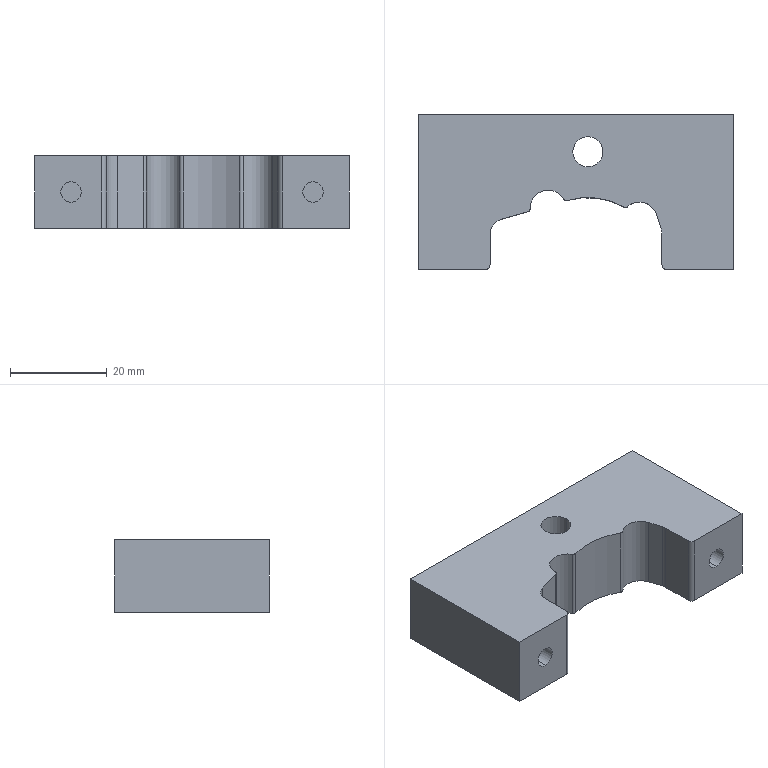NC program | Mastercam | posted with a generic post
Lines 1461 to 2481 of 2481:
N4690 T3 M6
N4700 G0 G90 G17 G54 X-12. Y-7.93 A0. S5500 M3
N4710 G43 H3 Z50.
N4720 Z2.
N4730 G1 Z-7.75 F2000.
N4740 X-12.829 Y-7.749 Z-7.901 F1500.
N4750 G3 X-13.069 Y-7.723 Z-7.944 I-.24 J-1.099
N4760 X-13.378 Y-7.766 Z-8. I0. J-1.125
N4770 G1 X-13.645 Y-7.842
N4780 G3 X-14.94 Y-8.789 I.372 J-1.868
N4790 X-15.116 Y-9.152 I2.014 J-1.201
N4800 X-15.15 Y-9.333 I.466 J-.181
N4810 G1 Y-9.519
N4820 Y-9.704
N4830 G3 X-14.22 Y-10.812 Z-7.75 I1.125 J0.
N4840 X-14.025 Y-10.829 I.195 J1.108 F9500.
N4850 X-13.15 Y-10.411 I0. J1.125
N4860 G1 X-12.537 Y-9.653
N4870 G3 X-12.287 Y-8.946 I-.875 J.707
N4880 X-12.4 Y-8.454 I-1.125 J0.
N4890 X-13.412 Y-7.821 Z-7.95 I-1.012 J-.492 F1500.
N4900 X-13.72 Y-7.864 Z-8. I0. J-1.125
N4910 G1 X-13.987 Y-7.94
N4920 G3 X-14.983 Y-8.648 I.375 J-1.582
N4930 X-15.088 Y-8.819 I1.467 J-1.022
N4940 X-15.15 Y-9.06 I.438 J-.241
N4950 G1 Y-9.245
N4960 Y-9.616
N4970 G3 X-14.22 Y-10.723 Z-7.75 I1.125 J0.
N4980 X-14.025 Y-10.74 I.195 J1.107 F9500.
N4990 X-13.102 Y-10.259 I0. J1.124
N5000 G1 X-12.671 Y-9.641
N5010 G3 X-12.469 Y-8.998 I-.923 J.643
N5020 X-12.582 Y-8.506 I-1.125 J0.
N5030 X-13.594 Y-7.873 Z-7.95 I-1.012 J-.492 F1500.
N5040 X-13.902 Y-7.916 Z-8. I0. J-1.125
N5050 G1 X-14.17 Y-7.992
N5060 G3 X-15.062 Y-8.589 I.257 J-1.348
N5070 X-15.15 Y-8.873 I.412 J-.284
N5080 G1 Y-9.058
N5090 Y-9.243
N5100 G3 X-14.22 Y-10.351 Z-7.75 I1.125 J0.
N5110 X-14.025 Y-10.368 I.195 J1.108 F9500.
N5120 X-13.265 Y-10.073 I0. J1.125
N5130 G1 X-13.07 Y-9.894
N5140 G3 X-12.705 Y-9.065 I-.76 J.829
N5150 X-12.819 Y-8.574 I-1.125 J0.
N5160 X-13.83 Y-7.941 Z-7.95 I-1.011 J-.491 F1500.
N5170 X-14.139 Y-7.983 Z-8. I0. J-1.124
N5180 G1 X-14.406 Y-8.059
N5190 G3 X-15.025 Y-8.412 I.199 J-1.068
N5200 X-15.15 Y-8.744 I.375 J-.332
N5210 G1 Y-8.929
N5220 Y-9.114
N5230 G3 X-14.22 Y-10.222 Z-7.75 I1.125 J0.
N5240 X-14.141 Y-10.233 I.195 J1.108 F9500.
N5250 X-14.009 Y-10.241 I.132 J1.117
N5260 X-12.884 Y-9.116 I0. J1.125
N5270 X-12.997 Y-8.624 I-1.125 J0.
N5280 X-14.009 Y-7.991 Z-7.95 I-1.012 J-.492 F1500.
N5290 X-14.317 Y-8.034 Z-8. I0. J-1.125
N5300 G1 X-14.584 Y-8.11
N5310 G3 X-14.882 Y-8.225 I.218 J-1.014
N5320 X-15.15 Y-8.724 I.332 J-.499
N5330 G1 Y-8.91
N5340 G3 X-14.22 Y-10.018 Z-7.75 I1.125 J0.
N5350 X-14.025 Y-10.035 I.195 J1.108 F9500.
N5360 X-13.603 Y-9.953 I0. J1.125
N5370 G1 X-3.746 Y-5.968
N5380 G3 X-3.109 Y-5.305 I-.422 J1.043
N5390 X-3.043 Y-4.925 Z-7.812 I-1.059 J.38 F1500.
N5400 X-3.61 Y-3.948 Z-8. I-1.125 J0.
N5410 G2 X-4.135 Y-3.586 I2.23 J3.793
N5420 G3 X-5.145 Y-3.338 I-1.01 J-1.933
N5430 X-5.937 Y-3.486 I0. J-2.181
N5440 X-6.878 Y-4.133 I.851 J-2.249
N5450 X-6.992 Y-4.334 I.366 J-.34
N5460 G2 X-7.049 Y-4.511 I-3.171 J.916
N5470 G3 X-7.112 Y-4.883 Z-7.94 I1.062 J-.372
N5480 X-6.538 Y-5.864 Z-7.75 I1.125 J0.
N5490 X-5.987 Y-6.008 I.551 J.981 F9500.
N5500 X-5.857 Y-6.001 I0. J1.125
N5510 G1 X-4.376 Y-5.829
N5520 G3 X-3.485 Y-5.185 I-.129 J1.118
N5530 X-3.38 Y-4.711 Z-7.828 I-1.02 J.474 F1500.
N5540 X-3.861 Y-3.789 Z-8. I-1.125 J0.
N5550 G2 X-4.262 Y-3.468 I1.729 J2.577
N5560 G3 X-5.198 Y-3.223 I-.936 J-1.662
N5570 X-5.612 Y-3.269 I0. J-1.907
N5580 X-6.806 Y-3.886 I.46 J-2.353
N5590 X-6.94 Y-4.131 I.354 J-.353
N5600 G2 X-6.986 Y-4.311 I-3.223 J.713
N5610 G3 X-7.028 Y-4.615 Z-7.951 I1.083 J-.304
N5620 X-6.39 Y-5.629 Z-7.75 I1.125 J0.
N5630 X-5.903 Y-5.74 I.487 J1.014 F9500.
N5640 X-5.854 Y-5.739 I0. J1.125
N5650 G1 X-4.656 Y-5.687
N5660 G3 X-3.713 Y-5.094 I-.049 J1.124
N5670 X-3.58 Y-4.563 Z-7.838 I-.992 J.531 F1500.
N5680 X-4.01 Y-3.679 Z-8. I-1.125 J0.
N5690 G2 X-4.397 Y-3.338 I2.158 J2.843
N5700 G3 X-5.27 Y-3.118 I-.873 J-1.622
N5710 X-5.649 Y-3.157 I0. J-1.842
N5720 X-6.76 Y-3.691 I.388 J-2.23
N5730 X-6.909 Y-3.97 I.344 J-.363
N5740 G2 X-6.945 Y-4.152 I-3.254 J.552
N5750 G3 X-6.973 Y-4.402 Z-7.96 I1.097 J-.25
N5760 X-6.285 Y-5.439 Z-7.75 I1.125 J0.
N5770 X-5.851 Y-5.527 I.437 J1.037 F9500.
N5780 G1 X-4.899 Y-5.529
N5790 X-4.896
N5800 G3 X-3.935 Y-4.99 I0. J1.125
N5810 X-3.77 Y-4.404 Z-7.848 I-.961 J.586 F1500.
N5820 X-4.153 Y-3.56 Z-8. I-1.126 J0.
N5830 G2 X-4.471 Y-3.252 I2.329 J2.723
N5840 G1 X-4.513 Y-3.224
N5850 G3 X-5.341 Y-3.014 I-.828 J-1.531
N5860 X-5.658 Y-3.043 I0. J-1.741
N5870 X-6.734 Y-3.528 I.277 J-2.05
N5880 X-6.888 Y-3.831 I.342 J-.365
N5890 G2 X-6.917 Y-4.014 I-3.275 J.413
N5900 G3 X-6.935 Y-4.217 Z-7.968 I1.107 J-.203
N5910 X-6.202 Y-5.271 Z-7.75 I1.125 J0.
N5920 X-5.922 Y-5.336 I.392 J1.054 F9500.
N5930 G1 X-5.126 Y-5.415
N5940 G3 X-5.015 Y-5.42 I.111 J1.119
N5950 X-4.076 Y-4.916 I0. J1.124
N5960 X-3.89 Y-4.296 Z-7.854 I-.939 J.62 F1500.
N5970 X-4.241 Y-3.479 Z-8. I-1.125 J0.
N5980 G2 X-4.55 Y-3.158 I2.414 J2.626
N5990 G1 X-4.589 Y-3.13
N6000 G3 X-5.415 Y-2.912 I-.826 J-1.456
N6010 X-5.699 Y-2.936 I0. J-1.674
N6020 X-6.722 Y-3.386 I.209 J-1.863
N6030 X-6.875 Y-3.705 I.345 J-.362
N6040 G2 X-6.928 Y-4.071 I-3.288 J.287
N6050 G3 X-6.95 Y-4.294 Z-7.964 I1.103 J-.223
N6060 X-6.236 Y-5.341 Z-7.75 I1.125 J0.
N6070 X-5.825 Y-5.419 I.411 J1.047 F9500.
N6080 X-5.64 Y-5.404 I0. J1.125
N6090 G1 X-4.949 Y-5.288
N6100 G3 X-4.219 Y-4.834 I-.185 J1.109
N6110 X-4.009 Y-4.179 Z-7.861 I-.915 J.655 F1500.
N6120 X-4.33 Y-3.392 Z-8. I-1.125 J0.
N6130 G2 X-4.614 Y-3.074 I2.538 J2.551
N6140 G1 X-4.65 Y-3.046
N6150 G3 X-5.482 Y-2.811 I-.832 J-1.356
N6160 X-5.721 Y-2.829 I0. J-1.591
N6170 X-6.712 Y-3.252 I.153 J-1.731
N6180 X-6.867 Y-3.589 I.344 J-.362
N6190 G2 X-6.907 Y-3.957 I-3.296 J.171
N6200 G3 X-6.922 Y-4.14 Z-7.971 I1.11 J-.183
N6210 X-6.17 Y-5.202 Z-7.75 I1.125 J0.
N6220 X-5.797 Y-5.266 I.373 J1.062 F9500.
N6230 X-5.663 Y-5.257 I0. J1.126
N6240 G1 X-5.1 Y-5.19
N6250 G3 X-4.342 Y-4.758 I-.134 J1.117
N6260 X-4.109 Y-4.073 Z-7.867 I-.892 J.685 F1500.
N6270 X-4.405 Y-3.313 Z-8. I-1.125 J0.
N6280 G2 X-4.677 Y-2.987 I2.534 J2.394
N6290 G1 X-4.711 Y-2.959
N6300 G3 X-5.544 Y-2.711 I-.833 J-1.276
N6310 X-5.747 Y-2.725 I0. J-1.524
N6320 X-6.723 Y-3.143 I.113 J-1.611
N6330 X-6.863 Y-3.481 I.36 J-.347
N6340 G2 X-6.891 Y-3.85 I-3.3 J.063
N6350 G3 X-6.901 Y-3.997 Z-7.977 I1.115 J-.147
N6360 X-6.114 Y-5.07 Z-7.75 I1.125 J0.
N6370 X-5.776 Y-5.122 I.338 J1.073 F9500.
N6380 X-5.693 Y-5.119 I0. J1.125
N6390 G1 X-5.247 Y-5.086
N6400 G3 X-4.461 Y-4.678 I-.083 J1.122
N6410 X-4.205 Y-3.964 Z-7.873 I-.869 J.714 F1500.
N6420 X-4.477 Y-3.232 Z-8. I-1.125 J0.
N6430 G2 X-4.733 Y-2.904 I2.56 J2.266
N6440 G1 X-4.765 Y-2.876
N6450 G3 X-5.614 Y-2.613 I-.849 J-1.239
N6460 X-5.849 Y-2.631 I0. J-1.502
N6470 X-6.721 Y-3.024 I.14 J-1.476
N6480 X-6.863 Y-3.373 I.358 J-.349
N6490 G1 Y-3.379
N6500 Y-3.418
N6510 G2 X-6.879 Y-3.749 I-3.3 J0.
N6520 G3 X-6.885 Y-3.861 Z-7.982 I1.119 J-.112
N6530 X-6.065 Y-4.944 Z-7.75 I1.125 J0.
N6540 X-5.76 Y-4.986 I.305 J1.083 F9500.
N6550 G1 X-5.754
N6560 X-5.412 Y-4.985
N6570 G3 X-4.57 Y-4.6 I-.005 J1.125
N6580 X-4.292 Y-3.86 Z-7.879 I-.847 J.74 F1500.
N6590 X-4.541 Y-3.154 Z-8. I-1.125 J0.
N6600 G2 X-4.786 Y-2.82 I2.721 J2.255
N6610 G1 X-4.817 Y-2.792
N6620 X-5.046 Y-2.648
N6630 G3 X-5.675 Y-2.519 I-.629 J-1.472
N6640 X-6.716 Y-2.904 I0. J-1.601
N6650 X-6.858 Y-3.206 I.355 J-.352
N6660 X-6.863 Y-3.315 I1.094 J-.109
N6670 G1 Y-3.341
N6680 G2 X-6.862 Y-3.418 I-3.3 J-.077
N6690 X-6.864 Y-3.526 I-3.301 J0.
N6700 G3 X-6.865 Y-3.563 Z-7.994 I1.124 J-.037
N6710 X-6.441 Y-4.443 Z-7.833 I1.125 J0.
N6720 G1 X-6.201 Y-4.634 Z-7.784
N6730 G3 X-6.019 Y-4.752 Z-7.75 I.701 J.88
N6740 X-5.5 Y-4.879 I.519 J.998 F9500.
N6750 X-4.675 Y-4.52 I0. J1.125
N6760 X-4.374 Y-3.754 Z-7.884 I-.825 J.766 F1500.
N6770 X-4.603 Y-3.075 Z-8. I-1.126 J0.
N6780 G2 X-4.835 Y-2.738 I2.854 J2.214
N6790 G1 X-4.864 Y-2.71
N6800 X-5.083 Y-2.564
N6810 G3 X-5.725 Y-2.426 I-.642 J-1.421
N6820 X-6.639 Y-2.721 I0. J-1.559
N6830 X-6.8 Y-2.946 I.31 J-.393
N6840 X-6.864 Y-3.315 I1.036 J-.369
N6850 X-6.863 Y-3.341 I1.1 J0.
N6860 G2 X-6.862 Y-3.418 I-3.3 J-.077
N6870 X-6.864 Y-3.526 I-3.301 J0.
N6880 G3 X-6.865 Y-3.563 Z-7.994 I1.124 J-.037
N6890 X-6.268 Y-4.556 Z-7.8 I1.125 J0.
N6900 G1 X-6.104 Y-4.643 Z-7.771
N6910 G3 X-5.985 Y-4.698 Z-7.75 I.528 J.993
N6920 X-5.576 Y-4.775 I.409 J1.048 F9500.
N6930 X-4.775 Y-4.439 I0. J1.125
N6940 X-4.452 Y-3.65 Z-7.889 I-.801 J.789 F1500.
N6950 X-4.66 Y-2.997 Z-8. I-1.124 J0.
N6960 G2 X-4.816 Y-2.757 I2.688 J1.914
N6970 G3 X-4.893 Y-2.643 I-.948 J-.558
N6980 G1 X-4.923 Y-2.614
N6990 X-5.146 Y-2.466
N7000 G3 X-5.77 Y-2.333 I-.624 J-1.393
N7010 X-6.46 Y-2.497 I0. J-1.526
N7020 X-6.627 Y-2.633 I.225 J-.446
N7030 X-6.849 Y-3.137 I.863 J-.682
N7040 X-6.862 Y-3.294 Z-7.975 I.956 J-.157
N7050 X-6.836 Y-3.517 Z-7.939 I.969 J0.
N7060 G1 X-6.782 Y-3.747 Z-7.901
N7070 G3 X-6.219 Y-4.479 Z-7.75 I1.095 J.26
N7080 X-5.687 Y-4.613 I.532 J.992 F9500.
N7090 X-4.921 Y-4.311 I0. J1.126
N7100 X-4.562 Y-3.487 Z-7.897 I-.766 J.824 F1500.
N7110 X-4.742 Y-2.876 Z-8. I-1.125 J0.
N7120 G2 X-4.816 Y-2.757 I2.77 J1.793
N7130 G3 X-5.118 Y-2.428 I-.891 J-.517
N7140 G1 X-5.163 Y-2.401
N7150 G3 X-5.801 Y-2.242 I-.638 J-1.204
N7160 X-6.174 Y-2.295 I0. J-1.363
N7170 X-6.721 Y-2.774 I.41 J-1.02
N7180 X-6.847 Y-3.251 Z-7.921 I.843 J-.477
N7190 X-6.311 Y-4.117 Z-7.75 I.969 J0.
N7200 X-5.878 Y-4.219 I.433 J.866 F9500.
N7210 X-5.834 Y-4.218 I0. J.968
N7220 X-5.757 Y-4.22 I.077 J1.271
N7230 X-5.146 Y-4.064 I0. J1.273
N7240 X-4.688 Y-3.241 Z-7.907 I-.51 J.823 F1500.
N7250 X-4.859 Y-2.69 Z-8. I-.968 J0.
N7260 X-5.764 Y-2.215 I-.905 J-.625
N7270 X-6.416 Y-2.429 I0. J-1.1
N7280 X-6.811 Y-3.21 Z-7.856 I.574 J-.781
N7290 X-6.592 Y-3.822 Z-7.75 I.969 J0.
N7300 X-6.051 Y-4.155 I.75 J.612 F9500.
N7310 G1 X13.364 Y-8.459
N7320 G3 X13.608 Y-8.486 I.244 J1.099
N7330 X14.133 Y-8.356 I0. J1.126
N7340 X14.734 Y-7.36 Z-7.944 I-.525 J.996 F1500.
N7350 X14.679 Y-7.016 Z-8. I-1.126 J0.
N7360 G1 X14.594 Y-6.752
N7370 G3 X13.611 Y-5.488 I-1.862 J-.434
N7380 X12.415 Y-5.199 I-1.196 J-2.332
N7390 X12.173 Y-5.21 I0. J-2.621
N7400 X11.96 Y-5.283 I.05 J-.498
N7410 G2 X11.8 Y-5.376 I-1.735 J2.807
N7420 G3 X11.212 Y-6.364 Z-7.808 I.537 J-.988
N7430 X11.27 Y-6.721 Z-7.75 I1.125 J0.
N7440 X11.783 Y-7.343 I1.067 J.357 F9500.
N7450 G1 X12.945 Y-8.
N7460 G3 X13.499 Y-8.146 I.554 J.979
N7470 X14.024 Y-8.016 I0. J1.125
N7480 X14.624 Y-7.021 Z-7.944 I-.525 J.995 F1500.
N7490 X14.57 Y-6.677 Z-8. I-1.125 J0.
N7500 G1 X14.485 Y-6.412
N7510 G3 X13.738 Y-5.433 I-1.574 J-.426
N7520 X12.456 Y-5.073 I-1.282 J-2.106
N7530 X12.409 Y-5.074 I0. J-2.466
N7540 X12.136 Y-5.166 I.016 J-.5
N7550 G2 X11.982 Y-5.269 I-1.911 J2.69
N7560 G3 X11.455 Y-6.222 Z-7.819 I.599 J-.953
N7570 X11.539 Y-6.646 Z-7.75 I1.126 J0.
N7580 X11.928 Y-7.138 I1.042 J.424 F9500.
N7590 G1 X12.786 Y-7.748
N7600 G3 X13.438 Y-7.956 I.652 J.916
N7610 X13.963 Y-7.827 I0. J1.124
N7620 X14.563 Y-6.832 Z-7.944 I-.525 J.995 F1500.
N7630 X14.509 Y-6.488 Z-8. I-1.125 J0.
N7640 G1 X14.424 Y-6.223
N7650 G3 X13.735 Y-5.309 I-1.403 J-.341
N7660 X12.566 Y-4.961 I-1.184 J-1.843
N7670 X12.267 Y-5.068 I.01 J-.5
N7680 G2 X12.118 Y-5.179 I-2.042 J2.592
N7690 G3 X11.639 Y-6.1 Z-7.828 I.645 J-.921
N7700 X11.744 Y-6.576 Z-7.75 I1.124 J0.
N7710 X12.04 Y-6.962 I1.019 J.476 F9500.
N7720 G1 X12.642 Y-7.468
N7730 G3 X13.365 Y-7.731 I.723 J.862
N7740 X13.89 Y-7.601 I0. J1.125
N7750 X14.49 Y-6.606 Z-7.944 I-.525 J.995 F1500.
N7760 X14.437 Y-6.262 Z-8. I-1.125 J0.
N7770 G1 X14.352 Y-5.997
N7780 G3 X13.769 Y-5.213 I-1.278 J-.341
N7790 X12.69 Y-4.86 I-1.11 J-1.569
N7800 X12.373 Y-4.98 I.009 J-.5
N7810 G2 X12.23 Y-5.097 I-2.148 J2.504
N7820 G3 X11.788 Y-5.991 Z-7.836 I.683 J-.894
N7830 X11.914 Y-6.509 Z-7.75 I1.125 J0.
N7840 X12.078 Y-6.744 I.999 J.518 F9500.
N7850 G1 X12.473 Y-7.183
N7860 G3 X13.309 Y-7.555 I.836 J.753
N7870 X13.834 Y-7.425 I0. J1.125
N7880 X14.434 Y-6.43 Z-7.944 I-.525 J.995 F1500.
N7890 X14.38 Y-6.086 Z-8. I-1.125 J0.
N7900 G1 X14.295 Y-5.821
N7910 G3 X14.143 Y-5.468 I-.983 J-.213
N7920 X12.837 Y-4.766 I-1.415 J-1.067
N7930 G1 X12.823
N7940 G3 X12.569 Y-4.835 I0. J-.5
N7950 X12.402 Y-4.956 I.558 J-.948
N7960 G2 X12.259 Y-5.074 I-2.177 J2.48
N7970 G3 X11.828 Y-5.96 Z-7.838 I.694 J-.886
N7980 X11.96 Y-6.489 Z-7.75 I1.125 J0.
N7990 X12.166 Y-6.764 I.993 J.529 F9500.
N8000 G1 X12.465 Y-7.057
N8010 G3 X13.252 Y-7.378 I.787 J.804
N8020 X13.777 Y-7.248 I0. J1.125
N8030 X14.377 Y-6.253 Z-7.944 I-.525 J.995 F1500.
N8040 X14.323 Y-5.909 Z-8. I-1.125 J0.
N8050 G1 X14.238 Y-5.645
N8060 X14.138 Y-5.383
N8070 G3 X13.14 Y-4.703 I-1.31 J-.852
N8080 X13.028 Y-4.69 I-.112 J-.488
N8090 X12.946 Y-4.698 I0. J-.501
N8100 X12.402 Y-4.956 I.181 J-1.085
N8110 G2 X12.259 Y-5.074 I-2.177 J2.48
N8120 G3 X11.828 Y-5.96 Z-7.838 I.694 J-.886
N8130 X11.96 Y-6.489 Z-7.75 I1.125 J0.
N8140 X12.465 Y-6.974 I.993 J.529 F9500.
N8150 G1 X12.708 Y-7.091
N8160 G3 X13.196 Y-7.202 I.488 J1.014
N8170 X13.72 Y-7.072 I0. J1.125
N8180 X14.321 Y-6.077 Z-7.944 I-.524 J.995 F1500.
N8190 X14.267 Y-5.733 Z-8. I-1.125 J0.
N8200 G1 X14.182 Y-5.468
N8210 G3 X13.127 Y-4.682 I-1.055 J-.315
N8220 X12.725 Y-4.759 I0. J-1.101
N8230 X12.11 Y-5.661 Z-7.815 I.354 J-.902
N8240 X12.197 Y-6.06 Z-7.75 I.969 J0.
N8250 X12.701 Y-6.553 I.882 J.399 F9500.
N8260 X13.238 Y-6.7 I.537 J.906
N8270 X13.575 Y-6.644 I0. J1.053
N8280 X14.217 Y-5.732 Z-7.939 I-.327 J.912 F1500.
N8290 X14.143 Y-5.359 Z-8. I-.969 J0.
N8300 X13.574 Y-4.777 I-1.016 J-.424
N8310 X13.181 Y-4.694 Z-7.936 I-.393 J-.886
N8320 X12.663 Y-4.844 Z-7.849 I0. J-.969
N8330 G1 X12.139 Y-5.175 Z-7.75
N8340 X10.346 Y-6.309 F9500.
N8350 G0 Z50.
N8360 X-12. Y-7.93
N8370 Z-6.
N8380 G1 Z-15.75 F2000.
N8390 X-12.829 Y-7.749 Z-15.901 F1500.
N8400 G3 X-13.069 Y-7.723 Z-15.944 I-.24 J-1.099
N8410 X-13.378 Y-7.766 Z-16. I0. J-1.125
N8420 G1 X-13.645 Y-7.842
N8430 G3 X-14.94 Y-8.789 I.372 J-1.868
N8440 X-15.116 Y-9.152 I2.014 J-1.201
N8450 X-15.15 Y-9.333 I.466 J-.181
N8460 G1 Y-9.519
N8470 Y-9.704
N8480 G3 X-14.22 Y-10.812 Z-15.75 I1.125 J0.
N8490 X-14.025 Y-10.829 I.195 J1.108 F9500.
N8500 X-13.15 Y-10.411 I0. J1.125
N8510 G1 X-12.537 Y-9.653
N8520 G3 X-12.287 Y-8.946 I-.875 J.707
N8530 X-12.4 Y-8.454 I-1.125 J0.
N8540 X-13.412 Y-7.821 Z-15.95 I-1.012 J-.492 F1500.
N8550 X-13.72 Y-7.864 Z-16. I0. J-1.125
N8560 G1 X-13.987 Y-7.94
N8570 G3 X-14.983 Y-8.648 I.375 J-1.582
N8580 X-15.088 Y-8.819 I1.467 J-1.022
N8590 X-15.15 Y-9.06 I.438 J-.241
N8600 G1 Y-9.245
N8610 Y-9.616
N8620 G3 X-14.22 Y-10.723 Z-15.75 I1.125 J0.
N8630 X-14.025 Y-10.74 I.195 J1.107 F9500.
N8640 X-13.102 Y-10.259 I0. J1.124
N8650 G1 X-12.671 Y-9.641
N8660 G3 X-12.469 Y-8.998 I-.923 J.643
N8670 X-12.582 Y-8.506 I-1.125 J0.
N8680 X-13.594 Y-7.873 Z-15.95 I-1.012 J-.492 F1500.
N8690 X-13.902 Y-7.916 Z-16. I0. J-1.125
N8700 G1 X-14.17 Y-7.992
N8710 G3 X-15.062 Y-8.589 I.257 J-1.348
N8720 X-15.15 Y-8.873 I.412 J-.284
N8730 G1 Y-9.058
N8740 Y-9.243
N8750 G3 X-14.22 Y-10.351 Z-15.75 I1.125 J0.
N8760 X-14.025 Y-10.368 I.195 J1.108 F9500.
N8770 X-13.265 Y-10.073 I0. J1.125
N8780 G1 X-13.07 Y-9.894
N8790 G3 X-12.705 Y-9.065 I-.76 J.829
N8800 X-12.819 Y-8.574 I-1.125 J0.
N8810 X-13.83 Y-7.941 Z-15.95 I-1.011 J-.491 F1500.
N8820 X-14.139 Y-7.983 Z-16. I0. J-1.124
N8830 G1 X-14.406 Y-8.059
N8840 G3 X-15.025 Y-8.412 I.199 J-1.068
N8850 X-15.15 Y-8.744 I.375 J-.332
N8860 G1 Y-8.929
N8870 Y-9.114
N8880 G3 X-14.22 Y-10.222 Z-15.75 I1.125 J0.
N8890 X-14.141 Y-10.233 I.195 J1.108 F9500.
N8900 X-14.009 Y-10.241 I.132 J1.117
N8910 X-12.884 Y-9.116 I0. J1.125
N8920 X-12.997 Y-8.624 I-1.125 J0.
N8930 X-14.009 Y-7.991 Z-15.95 I-1.012 J-.492 F1500.
N8940 X-14.317 Y-8.034 Z-16. I0. J-1.125
N8950 G1 X-14.584 Y-8.11
N8960 G3 X-14.882 Y-8.225 I.218 J-1.014
N8970 X-15.15 Y-8.724 I.332 J-.499
N8980 G1 Y-8.91
N8990 G3 X-14.22 Y-10.018 Z-15.75 I1.125 J0.
N9000 X-14.025 Y-10.035 I.195 J1.108 F9500.
N9010 X-13.603 Y-9.953 I0. J1.125
N9020 G1 X-3.746 Y-5.968
N9030 G3 X-3.109 Y-5.305 I-.422 J1.043
N9040 X-3.043 Y-4.925 Z-15.812 I-1.059 J.38 F1500.
N9050 X-3.61 Y-3.948 Z-16. I-1.125 J0.
N9060 G2 X-4.135 Y-3.586 I2.23 J3.793
N9070 G3 X-5.145 Y-3.338 I-1.01 J-1.933
N9080 X-5.937 Y-3.486 I0. J-2.181
N9090 X-6.878 Y-4.133 I.851 J-2.249
N9100 X-6.992 Y-4.334 I.366 J-.34
N9110 G2 X-7.049 Y-4.511 I-3.171 J.916
N9120 G3 X-7.112 Y-4.883 Z-15.94 I1.062 J-.372
N9130 X-6.538 Y-5.864 Z-15.75 I1.125 J0.
N9140 X-5.987 Y-6.008 I.551 J.981 F9500.
N9150 X-5.857 Y-6.001 I0. J1.125
N9160 G1 X-4.376 Y-5.829
N9170 G3 X-3.485 Y-5.185 I-.129 J1.118
N9180 X-3.38 Y-4.711 Z-15.828 I-1.02 J.474 F1500.
N9190 X-3.861 Y-3.789 Z-16. I-1.125 J0.
N9200 G2 X-4.262 Y-3.468 I1.729 J2.577
N9210 G3 X-5.198 Y-3.223 I-.936 J-1.662
N9220 X-5.612 Y-3.269 I0. J-1.907
N9230 X-6.806 Y-3.886 I.46 J-2.353
N9240 X-6.94 Y-4.131 I.354 J-.353
N9250 G2 X-6.986 Y-4.311 I-3.223 J.713
N9260 G3 X-7.028 Y-4.615 Z-15.951 I1.083 J-.304
N9270 X-6.39 Y-5.629 Z-15.75 I1.125 J0.
N9280 X-5.903 Y-5.74 I.487 J1.014 F9500.
N9290 X-5.854 Y-5.739 I0. J1.125
N9300 G1 X-4.656 Y-5.687
N9310 G3 X-3.713 Y-5.094 I-.049 J1.124
N9320 X-3.58 Y-4.563 Z-15.838 I-.992 J.531 F1500.
N9330 X-4.01 Y-3.679 Z-16. I-1.125 J0.
N9340 G2 X-4.397 Y-3.338 I2.158 J2.843
N9350 G3 X-5.27 Y-3.118 I-.873 J-1.622
N9360 X-5.649 Y-3.157 I0. J-1.842
N9370 X-6.76 Y-3.691 I.388 J-2.23
N9380 X-6.909 Y-3.97 I.344 J-.363
N9390 G2 X-6.945 Y-4.152 I-3.254 J.552
N9400 G3 X-6.973 Y-4.402 Z-15.96 I1.097 J-.25
N9410 X-6.285 Y-5.439 Z-15.75 I1.125 J0.
N9420 X-5.851 Y-5.527 I.437 J1.037 F9500.
N9430 G1 X-4.899 Y-5.529
N9440 X-4.896
N9450 G3 X-3.935 Y-4.99 I0. J1.125
N9460 X-3.77 Y-4.404 Z-15.848 I-.961 J.586 F1500.
N9470 X-4.153 Y-3.56 Z-16. I-1.126 J0.
N9480 G2 X-4.471 Y-3.252 I2.329 J2.723
N9490 G1 X-4.513 Y-3.224
N9500 G3 X-5.341 Y-3.014 I-.828 J-1.531
N9510 X-5.658 Y-3.043 I0. J-1.741
N9520 X-6.734 Y-3.528 I.277 J-2.05
N9530 X-6.888 Y-3.831 I.342 J-.365
N9540 G2 X-6.917 Y-4.014 I-3.275 J.413
N9550 G3 X-6.935 Y-4.217 Z-15.968 I1.107 J-.203
N9560 X-6.202 Y-5.271 Z-15.75 I1.125 J0.
N9570 X-5.922 Y-5.336 I.392 J1.054 F9500.
N9580 G1 X-5.126 Y-5.415
N9590 G3 X-5.015 Y-5.42 I.111 J1.119
N9600 X-4.076 Y-4.916 I0. J1.124
N9610 X-3.89 Y-4.296 Z-15.854 I-.939 J.62 F1500.
N9620 X-4.241 Y-3.479 Z-16. I-1.125 J0.
N9630 G2 X-4.55 Y-3.158 I2.414 J2.626
N9640 G1 X-4.589 Y-3.13
N9650 G3 X-5.415 Y-2.912 I-.826 J-1.456
N9660 X-5.699 Y-2.936 I0. J-1.674
N9670 X-6.722 Y-3.386 I.209 J-1.863
N9680 X-6.875 Y-3.705 I.345 J-.362
N9690 G2 X-6.928 Y-4.071 I-3.288 J.287
N9700 G3 X-6.95 Y-4.294 Z-15.964 I1.103 J-.223
N9710 X-6.236 Y-5.341 Z-15.75 I1.125 J0.
N9720 X-5.825 Y-5.419 I.411 J1.047 F9500.
N9730 X-5.64 Y-5.404 I0. J1.125
N9740 G1 X-4.949 Y-5.288
N9750 G3 X-4.219 Y-4.834 I-.185 J1.109
N9760 X-4.009 Y-4.179 Z-15.861 I-.915 J.655 F1500.
N9770 X-4.33 Y-3.392 Z-16. I-1.125 J0.
N9780 G2 X-4.614 Y-3.074 I2.538 J2.551
N9790 G1 X-4.65 Y-3.046
N9800 G3 X-5.482 Y-2.811 I-.832 J-1.356
N9810 X-5.721 Y-2.829 I0. J-1.591
N9820 X-6.712 Y-3.252 I.153 J-1.731
N9830 X-6.867 Y-3.589 I.344 J-.362
N9840 G2 X-6.907 Y-3.957 I-3.296 J.171
N9850 G3 X-6.922 Y-4.14 Z-15.971 I1.11 J-.183
N9860 X-6.17 Y-5.202 Z-15.75 I1.125 J0.
N9870 X-5.797 Y-5.266 I.373 J1.062 F9500.
N9880 X-5.663 Y-5.257 I0. J1.126
N9890 G1 X-5.1 Y-5.19
N9900 G3 X-4.342 Y-4.758 I-.134 J1.117
N9910 X-4.109 Y-4.073 Z-15.867 I-.892 J.685 F1500.
N9920 X-4.405 Y-3.313 Z-16. I-1.125 J0.
N9930 G2 X-4.677 Y-2.987 I2.534 J2.394
N9940 G1 X-4.711 Y-2.959
N9950 G3 X-5.544 Y-2.711 I-.833 J-1.276
N9960 X-5.747 Y-2.725 I0. J-1.524
N9970 X-6.723 Y-3.143 I.113 J-1.611
N9980 X-6.863 Y-3.481 I.36 J-.347
N9990 G2 X-6.891 Y-3.85 I-3.3 J.063
N100 G3 X-6.901 Y-3.997 Z-15.977 I1.115 J-.147
N110 X-6.114 Y-5.07 Z-15.75 I1.125 J0.
N120 X-5.776 Y-5.122 I.338 J1.073 F9500.
N130 X-5.693 Y-5.119 I0. J1.125
N140 G1 X-5.247 Y-5.086
N150 G3 X-4.461 Y-4.678 I-.083 J1.122
N160 X-4.205 Y-3.964 Z-15.873 I-.869 J.714 F1500.
N170 X-4.477 Y-3.232 Z-16. I-1.125 J0.
N180 G2 X-4.733 Y-2.904 I2.56 J2.266
N190 G1 X-4.765 Y-2.876
N200 G3 X-5.614 Y-2.613 I-.849 J-1.239
N210 X-5.849 Y-2.631 I0. J-1.502
N220 X-6.721 Y-3.024 I.14 J-1.476
N230 X-6.863 Y-3.373 I.358 J-.349
N240 G1 Y-3.379
N250 Y-3.418
N260 G2 X-6.879 Y-3.749 I-3.3 J0.
N270 G3 X-6.885 Y-3.861 Z-15.982 I1.119 J-.112
N280 X-6.065 Y-4.944 Z-15.75 I1.125 J0.
N290 X-5.76 Y-4.986 I.305 J1.083 F9500.
N300 G1 X-5.754
N310 X-5.412 Y-4.985
N320 G3 X-4.57 Y-4.6 I-.005 J1.125
N330 X-4.292 Y-3.86 Z-15.879 I-.847 J.74 F1500.
N340 X-4.541 Y-3.154 Z-16. I-1.125 J0.
N350 G2 X-4.786 Y-2.82 I2.721 J2.255
N360 G1 X-4.817 Y-2.792
N370 X-5.046 Y-2.648
N380 G3 X-5.675 Y-2.519 I-.629 J-1.472
N390 X-6.716 Y-2.904 I0. J-1.601
N400 X-6.858 Y-3.206 I.355 J-.352
N410 X-6.863 Y-3.315 I1.094 J-.109
N420 G1 Y-3.341
N430 G2 X-6.862 Y-3.418 I-3.3 J-.077
N440 X-6.864 Y-3.526 I-3.301 J0.
N450 G3 X-6.865 Y-3.563 Z-15.994 I1.124 J-.037
N460 X-6.441 Y-4.443 Z-15.833 I1.125 J0.
N470 G1 X-6.201 Y-4.634 Z-15.784
N480 G3 X-6.019 Y-4.752 Z-15.75 I.701 J.88
N490 X-5.5 Y-4.879 I.519 J.998 F9500.
N500 X-4.675 Y-4.52 I0. J1.125
N510 X-4.374 Y-3.754 Z-15.884 I-.825 J.766 F1500.
N520 X-4.603 Y-3.075 Z-16. I-1.126 J0.
N530 G2 X-4.835 Y-2.738 I2.854 J2.214
N540 G1 X-4.864 Y-2.71
N550 X-5.083 Y-2.564
N560 G3 X-5.725 Y-2.426 I-.642 J-1.421
N570 X-6.639 Y-2.721 I0. J-1.559
N580 X-6.8 Y-2.946 I.31 J-.393
N590 X-6.864 Y-3.315 I1.036 J-.369
N600 X-6.863 Y-3.341 I1.1 J0.
N610 G2 X-6.862 Y-3.418 I-3.3 J-.077
N620 X-6.864 Y-3.526 I-3.301 J0.
N630 G3 X-6.865 Y-3.563 Z-15.994 I1.124 J-.037
N640 X-6.268 Y-4.556 Z-15.8 I1.125 J0.
N650 G1 X-6.104 Y-4.643 Z-15.771
N660 G3 X-5.985 Y-4.698 Z-15.75 I.528 J.993
N670 X-5.576 Y-4.775 I.409 J1.048 F9500.
N680 X-4.775 Y-4.439 I0. J1.125
N690 X-4.452 Y-3.65 Z-15.889 I-.801 J.789 F1500.
N700 X-4.66 Y-2.997 Z-16. I-1.124 J0.
N710 G2 X-4.816 Y-2.757 I2.688 J1.914
N720 G3 X-4.893 Y-2.643 I-.948 J-.558
N730 G1 X-4.923 Y-2.614
N740 X-5.146 Y-2.466
N750 G3 X-5.77 Y-2.333 I-.624 J-1.393
N760 X-6.46 Y-2.497 I0. J-1.526
N770 X-6.627 Y-2.633 I.225 J-.446
N780 X-6.849 Y-3.137 I.863 J-.682
N790 X-6.862 Y-3.294 Z-15.975 I.956 J-.157
N800 X-6.836 Y-3.517 Z-15.939 I.969 J0.
N810 G1 X-6.782 Y-3.747 Z-15.901
N820 G3 X-6.219 Y-4.479 Z-15.75 I1.095 J.26
N830 X-5.687 Y-4.613 I.532 J.992 F9500.
N840 X-4.921 Y-4.311 I0. J1.126
N850 X-4.562 Y-3.487 Z-15.897 I-.766 J.824 F1500.
N860 X-4.742 Y-2.876 Z-16. I-1.125 J0.
N870 G2 X-4.816 Y-2.757 I2.77 J1.793
N880 G3 X-5.118 Y-2.428 I-.891 J-.517
N890 G1 X-5.163 Y-2.401
N900 G3 X-5.801 Y-2.242 I-.638 J-1.204
N910 X-6.174 Y-2.295 I0. J-1.363
N920 X-6.721 Y-2.774 I.41 J-1.02
N930 X-6.847 Y-3.251 Z-15.921 I.843 J-.477
N940 X-6.311 Y-4.117 Z-15.75 I.969 J0.
N950 X-5.878 Y-4.219 I.433 J.866 F9500.
N960 X-5.834 Y-4.218 I0. J.968
N970 X-5.757 Y-4.22 I.077 J1.271
N980 X-5.146 Y-4.064 I0. J1.273
N990 X-4.688 Y-3.241 Z-15.907 I-.51 J.823 F1500.
N1000 X-4.859 Y-2.69 Z-16. I-.968 J0.
N1010 X-5.764 Y-2.215 I-.905 J-.625
N1020 X-6.416 Y-2.429 I0. J-1.1
N1030 X-6.811 Y-3.21 Z-15.856 I.574 J-.781
N1040 X-6.592 Y-3.822 Z-15.75 I.969 J0.
N1050 X-6.051 Y-4.155 I.75 J.612 F9500.
N1060 G1 X13.364 Y-8.459
N1070 G3 X13.608 Y-8.486 I.244 J1.099
N1080 X14.133 Y-8.356 I0. J1.126
N1090 X14.734 Y-7.36 Z-15.944 I-.525 J.996 F1500.
N1100 X14.679 Y-7.016 Z-16. I-1.126 J0.
N1110 G1 X14.594 Y-6.752
N1120 G3 X13.611 Y-5.488 I-1.862 J-.434
N1130 X12.415 Y-5.199 I-1.196 J-2.332
N1140 X12.173 Y-5.21 I0. J-2.621
N1150 X11.96 Y-5.283 I.05 J-.498
N1160 G2 X11.8 Y-5.376 I-1.735 J2.807
N1170 G3 X11.212 Y-6.364 Z-15.808 I.537 J-.988
N1180 X11.27 Y-6.721 Z-15.75 I1.125 J0.
N1190 X11.783 Y-7.343 I1.067 J.357 F9500.
N1200 G1 X12.945 Y-8.
N1210 G3 X13.499 Y-8.146 I.554 J.979
N1220 X14.024 Y-8.016 I0. J1.125
N1230 X14.624 Y-7.021 Z-15.944 I-.525 J.995 F1500.
N1240 X14.57 Y-6.677 Z-16. I-1.125 J0.
N1250 G1 X14.485 Y-6.412
N1260 G3 X13.738 Y-5.433 I-1.574 J-.426
N1270 X12.456 Y-5.073 I-1.282 J-2.106
N1280 X12.409 Y-5.074 I0. J-2.466
N1290 X12.136 Y-5.166 I.016 J-.5
N1300 G2 X11.982 Y-5.269 I-1.911 J2.69
N1310 G3 X11.455 Y-6.222 Z-15.819 I.599 J-.953
N1320 X11.539 Y-6.646 Z-15.75 I1.126 J0.
N1330 X11.928 Y-7.138 I1.042 J.424 F9500.
N1340 G1 X12.786 Y-7.748
N1350 G3 X13.438 Y-7.956 I.652 J.916
N1360 X13.963 Y-7.827 I0. J1.124
N1370 X14.563 Y-6.832 Z-15.944 I-.525 J.995 F1500.
N1380 X14.509 Y-6.488 Z-16. I-1.125 J0.
N1390 G1 X14.424 Y-6.223
N1400 G3 X13.735 Y-5.309 I-1.403 J-.341
N1410 X12.566 Y-4.961 I-1.184 J-1.843
N1420 X12.267 Y-5.068 I.01 J-.5
N1430 G2 X12.118 Y-5.179 I-2.042 J2.592
N1440 G3 X11.639 Y-6.1 Z-15.828 I.645 J-.921
N1450 X11.744 Y-6.576 Z-15.75 I1.124 J0.
N1460 X12.04 Y-6.962 I1.019 J.476 F9500.
N1470 G1 X12.642 Y-7.468
N1480 G3 X13.365 Y-7.731 I.723 J.862
N1490 X13.89 Y-7.601 I0. J1.125
N1500 X14.49 Y-6.606 Z-15.944 I-.525 J.995 F1500.
N1510 X14.437 Y-6.262 Z-16. I-1.125 J0.
N1520 G1 X14.352 Y-5.997
N1530 G3 X13.769 Y-5.213 I-1.278 J-.341
N1540 X12.69 Y-4.86 I-1.11 J-1.569
N1550 X12.373 Y-4.98 I.009 J-.5
N1560 G2 X12.23 Y-5.097 I-2.148 J2.504
N1570 G3 X11.788 Y-5.991 Z-15.836 I.683 J-.894
N1580 X11.914 Y-6.509 Z-15.75 I1.125 J0.
N1590 X12.078 Y-6.744 I.999 J.518 F9500.
N1600 G1 X12.473 Y-7.183
N1610 G3 X13.309 Y-7.555 I.836 J.753
N1620 X13.834 Y-7.425 I0. J1.125
N1630 X14.434 Y-6.43 Z-15.944 I-.525 J.995 F1500.
N1640 X14.38 Y-6.086 Z-16. I-1.125 J0.
N1650 G1 X14.295 Y-5.821
N1660 G3 X14.143 Y-5.468 I-.983 J-.213
N1670 X12.837 Y-4.766 I-1.415 J-1.067
N1680 G1 X12.823
N1690 G3 X12.569 Y-4.835 I0. J-.5
N1700 X12.402 Y-4.956 I.558 J-.948
N1710 G2 X12.259 Y-5.074 I-2.177 J2.48
N1720 G3 X11.828 Y-5.96 Z-15.838 I.694 J-.886
N1730 X11.96 Y-6.489 Z-15.75 I1.125 J0.
N1740 X12.166 Y-6.764 I.993 J.529 F9500.
N1750 G1 X12.465 Y-7.057
N1760 G3 X13.252 Y-7.378 I.787 J.804
N1770 X13.777 Y-7.248 I0. J1.125
N1780 X14.377 Y-6.253 Z-15.944 I-.525 J.995 F1500.
N1790 X14.323 Y-5.909 Z-16. I-1.125 J0.
N1800 G1 X14.238 Y-5.645
N1810 X14.138 Y-5.383
N1820 G3 X13.14 Y-4.703 I-1.31 J-.852
N1830 X13.028 Y-4.69 I-.112 J-.488
N1840 X12.946 Y-4.698 I0. J-.501
N1850 X12.402 Y-4.956 I.181 J-1.085
N1860 G2 X12.259 Y-5.074 I-2.177 J2.48
N1870 G3 X11.828 Y-5.96 Z-15.838 I.694 J-.886
N1880 X11.96 Y-6.489 Z-15.75 I1.125 J0.
N1890 X12.465 Y-6.974 I.993 J.529 F9500.
N1900 G1 X12.708 Y-7.091
N1910 G3 X13.196 Y-7.202 I.488 J1.014
N1920 X13.72 Y-7.072 I0. J1.125
N1930 X14.321 Y-6.077 Z-15.944 I-.524 J.995 F1500.
N1940 X14.267 Y-5.733 Z-16. I-1.125 J0.
N1950 G1 X14.182 Y-5.468
N1960 G3 X13.127 Y-4.682 I-1.055 J-.315
N1970 X12.725 Y-4.759 I0. J-1.101
N1980 X12.11 Y-5.661 Z-15.815 I.354 J-.902
N1990 X12.197 Y-6.06 Z-15.75 I.969 J0.
N2000 X12.701 Y-6.553 I.882 J.399 F9500.
N2010 X13.238 Y-6.7 I.537 J.906
N2020 X13.575 Y-6.644 I0. J1.053
N2030 X14.217 Y-5.732 Z-15.939 I-.327 J.912 F1500.
N2040 X14.143 Y-5.359 Z-16. I-.969 J0.
N2050 X13.574 Y-4.777 I-1.016 J-.424
N2060 X13.181 Y-4.694 Z-15.936 I-.393 J-.886
N2070 X12.663 Y-4.844 Z-15.849 I0. J-.969
N2080 G1 X12.139 Y-5.175 Z-15.75
N2090 X10.346 Y-6.309 F9500.
N2100 G0 Z50.
N2110 M5
N2120 G91 G28 Z0.
N2130 A0.
N2140 M01
N2150 T5 M6
N2160 G0 G90 G17 G54 X2.45 Y8.3 A0. S3000 M3
N2170 G43 H5 Z50.
N2180 G98 G81 Z-3.1 R1. F300.
N2190 G80
N2200 M5
N2210 G91 G0 G28 Z0.
N2220 A0.
N2230 M01
N2240 T11 M6
N2250 G0 G90 G17 G54 X2.45 Y8.3 A0. S3000 M3
N2260 G43 H11 Z50.
N2270 G98 G83 Z-20. R1. Q4. F300.
N2280 G80
N2290 M5
N2300 G91 G0 G28 Z0.
N2310 A0.
N2320 M01
N2330 T5 M6
N2340 G0 G90 G17 G54 X32.9 Y-19.5 A0. S5000 M3
N2350 G43 H5 Z50.
N2360 Z1.
N2370 G1 Z-1.1 F2000.
N2380 G41 D5 Y-17.5 F1000.
N2390 G3 X32.4 Y-17. I-.5 J0.
N2400 G1 X18.745
N2410 G2 X16.745 Y-15. I0. J2.
N2420 G1 Y-8.53
N2430 G3 X16.649 Y-7.918 I-2. J0.
N2440 G1 X15.698 Y-4.957
N2450 G3 X13.127 Y-3.083 I-2.571 J-.826
N2460 X11.346 Y-3.754 I0. J-2.7
N2470 G2 X10.225 Y-4.176 I-1.121 J1.278
N2480 X9.399 Y-3.962 I0. J1.7
N2490 G3 X2.45 Y-2.16 I-6.949 J-12.498
N2500 X-1.502 Y-2.717 I0. J-14.3
N2510 G2 X-1.972 Y-2.783 I-.47 J1.634
N2520 X-3.437 Y-1.946 I0. J1.7
N2530 G3 X-5.764 Y-.615 I-2.327 J-1.369
N2540 X-8.464 Y-3.315 I0. J-2.7
N2550 X-8.463 Y-3.379 I2.7 J0.
N2560 G1 Y-3.418
N2570 G2 X-9.697 Y-5.053 I-1.7 J0.
N2580 G1 X-15.153 Y-6.609
N2590 G3 X-16.75 Y-8.724 I.603 J-2.115
N2600 G1 Y-15.
N2610 G2 X-18.75 Y-17. I-2. J0.
N2620 G1 X-32.4
N2630 G2 X-33.5 Y-15.9 I0. J1.1
N2640 G1 Y15.9
N2650 G2 X-32.4 Y17. I1.1 J0.
N2660 G1 X32.4
N2670 G2 X33.5 Y15.9 I0. J-1.1
N2680 G1 Y-15.9
N2690 G2 X32.4 Y-17. I-1.1 J0.
N2700 G1 X31.9
N2710 G3 X31.4 Y-17.5 I0. J-.5
N2720 G1 G40 Y-19.5
N2730 G0 Z50.
N2740 M5
N2750 G91 G28 Z0.
N2760 A0.
N2770 M01
N2780 T10 M6
N2790 G0 G90 G17 G54 X32.9 Y-23.5 A0. S5000 M3
N2800 G43 H10 Z50.
N2810 Z1.
N2820 G1 Z-16. F2000.
N2830 G41 D10 Y-20.5 F600.
N2840 G3 X32.4 Y-20. I-.5 J0.
N2850 G1 X18.745
N2860 G2 X13.745 Y-15. I0. J5.
N2870 G1 Y-8.687
N2880 X12.974 Y-6.288
N2890 G2 X10.225 Y-7.176 I-2.749 J3.812
N2900 X7.941 Y-6.584 I0. J4.7
N2910 G3 X2.45 Y-5.16 I-5.491 J-9.876
N2920 X-.673 Y-5.6 I0. J-11.3
N2930 G2 X-1.972 Y-5.783 I-1.299 J4.517
N2940 X-5.522 Y-4.163 I0. J4.7
N2950 X-8.874 Y-7.938 I-4.641 J.745
N2960 G1 X-13.75 Y-9.328
N2970 Y-15.
N2980 G2 X-18.75 Y-20. I-5. J0.
N2990 G1 X-32.4
N3000 G2 X-36.5 Y-15.9 I0. J4.1
N3010 G1 Y15.9
N3020 G2 X-32.4 Y20. I4.1 J0.
N3030 G1 X32.4
N3040 G2 X36.5 Y15.9 I0. J-4.1
N3050 G1 Y-15.9
N3060 G2 X32.4 Y-20. I-4.1 J0.
N3070 G1 X31.9
N3080 G3 X31.4 Y-20.5 I0. J-.5
N3090 G1 G40 Y-23.5
N3100 X32.9
N3110 G41 D10 Y-20.5
N3120 G3 X32.4 Y-20. I-.5 J0.
N3130 G1 X18.745
N3140 G2 X13.745 Y-15. I0. J5.
N3150 G1 Y-8.687
N3160 X12.974 Y-6.288
N3170 G2 X10.225 Y-7.176 I-2.749 J3.812
N3180 X7.941 Y-6.584 I0. J4.7
N3190 G3 X2.45 Y-5.16 I-5.491 J-9.876
N3200 X-.673 Y-5.6 I0. J-11.3
N3210 G2 X-1.972 Y-5.783 I-1.299 J4.517
N3220 X-5.522 Y-4.163 I0. J4.7
N3230 X-8.874 Y-7.938 I-4.641 J.745
N3240 G1 X-13.75 Y-9.328
N3250 Y-15.
N3260 G2 X-18.75 Y-20. I-5. J0.
N3270 G1 X-32.4
N3280 G2 X-36.5 Y-15.9 I0. J4.1
N3290 G1 Y15.9
N3300 G2 X-32.4 Y20. I4.1 J0.
N3310 G1 X32.4
N3320 G2 X36.5 Y15.9 I0. J-4.1
N3330 G1 Y-15.9
N3340 G2 X32.4 Y-20. I-4.1 J0.
N3350 G1 X31.9
N3360 G3 X31.4 Y-20.5 I0. J-.5
N3370 G1 G40 Y-23.5
N3380 G0 Z50.
N3390 M5
N3400 G91 G28 Z0.
N3410 A0.
N3420 M01
N3430 T3 M6
N3440 G0 G90 G17 G54 X15.245 Y-18. A0. S5000 M3
N3450 G43 H3 Z50.
N3460 Z1.
N3470 G1 Z-15.2 F2000.
N3480 G41 D3 Y-15. F600.
N3490 Y-8.53
N3500 G3 X15.221 Y-8.377 I-.5 J0.
N3510 G1 X14.27 Y-5.416
N3520 G3 X13.127 Y-4.583 I-1.143 J-.367
N3530 X12.336 Y-4.881 I0. J-1.2
N3540 G2 X10.225 Y-5.676 I-2.111 J2.405
N3550 X8.67 Y-5.273 I0. J3.2
N3560 G3 X2.45 Y-3.66 I-6.22 J-11.187
N3570 X-1.088 Y-4.159 I0. J-12.8
N3580 G2 X-1.972 Y-4.284 I-.884 J3.076
N3590 X-4.73 Y-2.707 I0. J3.201
N3600 G3 X-5.764 Y-2.115 I-1.034 J-.608
N3610 X-6.964 Y-3.315 I0. J-1.2
N3620 X-6.963 Y-3.343 I1.2 J0.
N3630 G2 X-6.962 Y-3.418 I-3.2 J-.075
N3640 X-9.285 Y-6.496 I-3.201 J0.
N3650 G1 X-14.742 Y-8.051
N3660 G3 X-15.25 Y-8.724 I.192 J-.673
N3670 G1 Y-15.
N3680 G40 Y-18.
N3690 G0 Z50.
N3700 X15.245
N3710 Z1.
N3720 G1 Z-15.2 F2000.
N3730 G41 D3 Y-15. F600.
N3740 Y-8.53
N3750 G3 X15.221 Y-8.377 I-.5 J0.
N3760 G1 X14.27 Y-5.416
N3770 G3 X13.127 Y-4.583 I-1.143 J-.367
N3780 X12.336 Y-4.881 I0. J-1.2
N3790 G2 X10.225 Y-5.676 I-2.111 J2.405
N3800 X8.67 Y-5.273 I0. J3.2
N3810 G3 X2.45 Y-3.66 I-6.22 J-11.187
N3820 X-1.088 Y-4.159 I0. J-12.8
N3830 G2 X-1.972 Y-4.284 I-.884 J3.076
N3840 X-4.73 Y-2.707 I0. J3.201
N3850 G3 X-5.764 Y-2.115 I-1.034 J-.608
N3860 X-6.964 Y-3.315 I0. J-1.2
N3870 X-6.963 Y-3.343 I1.2 J0.
N3880 G2 X-6.962 Y-3.418 I-3.2 J-.075
N3890 X-9.285 Y-6.496 I-3.201 J0.
N3900 G1 X-14.742 Y-8.051
N3910 G3 X-15.25 Y-8.724 I.192 J-.673
N3920 G1 Y-15.
N3930 G40 Y-18.
N3940 G0 Z50.
N3950 M5
N3960 G91 G28 Z0.
N3970 A0.
N3980 M01
N3990 T1 M6
N4000 G0 G90 G17 G55 X75. Y0. A180. S5000 M3
N4010 G43 H1 Z50.
N4020 Z7.
N4030 G1 Z4.02 F2000.
N4040 X-75. F1500.
N4050 Z3.04 F2000.
N4060 X75. F1500.
N4070 Z2.06 F2000.
N4080 X-75. F1500.
N4090 Z1.08 F2000.
N4100 X75. F1500.
N4110 Z.1 F2000.
N4120 X-75. F1500.
N4130 G0 Z50.
N4140 X75.
N4150 Z2.
N4160 G1 Z0. F2000.
N4170 X-75. F700.
N4180 G0 Z50.
N4190 M5
N4200 G91 G28 Z0.
N4210 A0.
N4220 M01
N4230 T5 M6
N4240 G0 G90 G17 G55 X-2.45 Y8.3 A180. S3000 M3
N4250 G43 H5 Z50.
N4260 G98 G81 Z-3.1 R1. F400.
N4270 G80
N4280 S5000 M3
N4290 G0 X32.9 Y-19.5
N4300 Z1.
N4310 G1 Z-1.2 F2000.
N4320 G41 D5 Y-17.5 F1000.
N4330 G3 X32.4 Y-17. I-.5 J0.
N4340 G1 X18.75
N4350 G2 X16.75 Y-15. I0. J2.
N4360 G1 Y-8.724
N4370 G3 X15.153 Y-6.609 I-2.2 J0.
N4380 G1 X9.697 Y-5.053
N4390 G2 X8.463 Y-3.418 I.466 J1.635
N4400 G1 Y-3.379
N4410 G3 X8.464 Y-3.315 I-2.699 J.064
N4420 X5.764 Y-.615 I-2.7 J0.
N4430 X3.437 Y-1.946 I0. J-2.7
N4440 G2 X1.972 Y-2.783 I-1.465 J.863
N4450 X1.502 Y-2.717 I0. J1.7
N4460 G3 X-2.45 Y-2.16 I-3.952 J-13.743
N4470 X-9.399 Y-3.962 I0. J-14.3
N4480 G2 X-10.225 Y-4.176 I-.826 J1.486
N4490 X-11.346 Y-3.754 I0. J1.7
N4500 G3 X-13.127 Y-3.083 I-1.781 J-2.029
N4510 X-15.698 Y-4.957 I0. J-2.7
N4520 G1 X-16.649 Y-7.918
N4530 G3 X-16.745 Y-8.53 I1.904 J-.612
N4540 G1 Y-15.
N4550 G2 X-18.745 Y-17. I-2. J0.
N4560 G1 X-32.4
N4570 G2 X-33.5 Y-15.9 I0. J1.1
N4580 G1 Y15.9
N4590 G2 X-32.4 Y17. I1.1 J0.
N4600 G1 X32.4
N4610 G2 X33.5 Y15.9 I0. J-1.1
N4620 G1 Y-15.9
N4630 G2 X32.4 Y-17. I-1.1 J0.
N4640 G1 X31.9
N4650 G3 X31.4 Y-17.5 I0. J-.5
N4660 G1 G40 Y-19.5
N4670 G0 Z50.
N4680 S3000 M3
N4690 G56 X-25. Y0. Z50. A270.
N4700 G98 G81 Z-2. R1. F300.
N4710 X25.
N4720 G80
N4730 M5
N4740 G91 G0 G28 Z0.
N4750 A0.
N4760 M01
N4770 T15 M6
N4780 G0 G90 G17 G56 X-25. Y0. A-90. S3000 M3
N4790 G43 H15 Z50.
N4800 G98 G83 Z-16. R1. Q2. F300.
N4810 X25.
N4820 G80
N4830 M5
N4840 G91 G0 G28 Z0.
N4850 A0.
N4860 M01
N4870 T16 M6
N4880 G0 G90 G17 G56 X-25. Y0. A-90. S400 M3
N4890 G43 H16 Z50.
N4900 G94
N4910 G98 G84 Z-12. R1. F320.
N4920 X25.
N4930 G80
N4940 G94
N4950 M5
N4960 G91 G0 G28 Z0.
N4970 G28 X0. Y0. A0.
N4980 M30
%